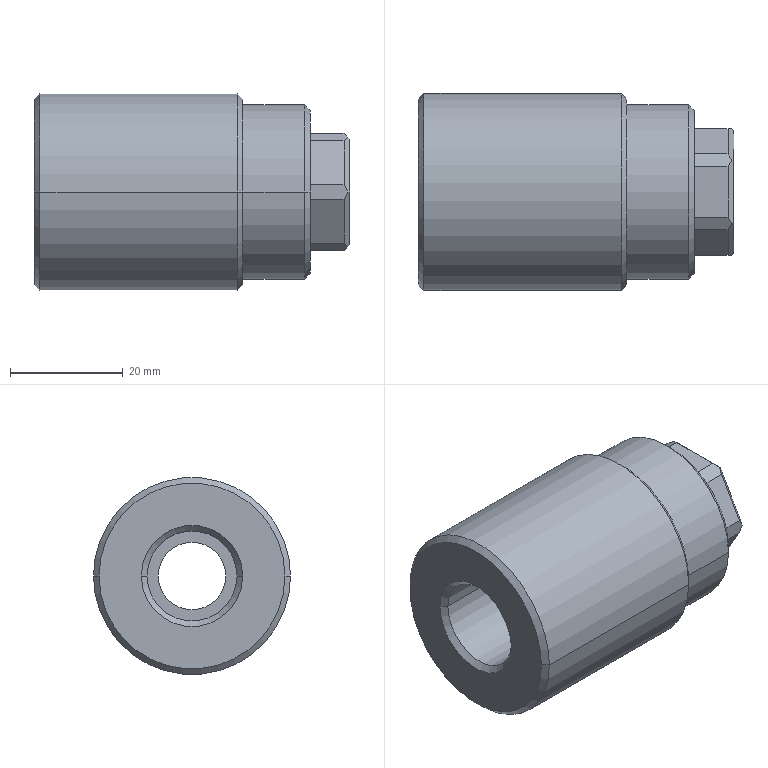Part | STEP file | PN_0018 | 1 solid | 41 faces | box 56 x 35 x 35 mm | volume 37589 mm3 | plane 23 | cone 10 | cylinder 8 | commonest cylinder face diameters 12 x2 16 x2 31 x2 35 x2